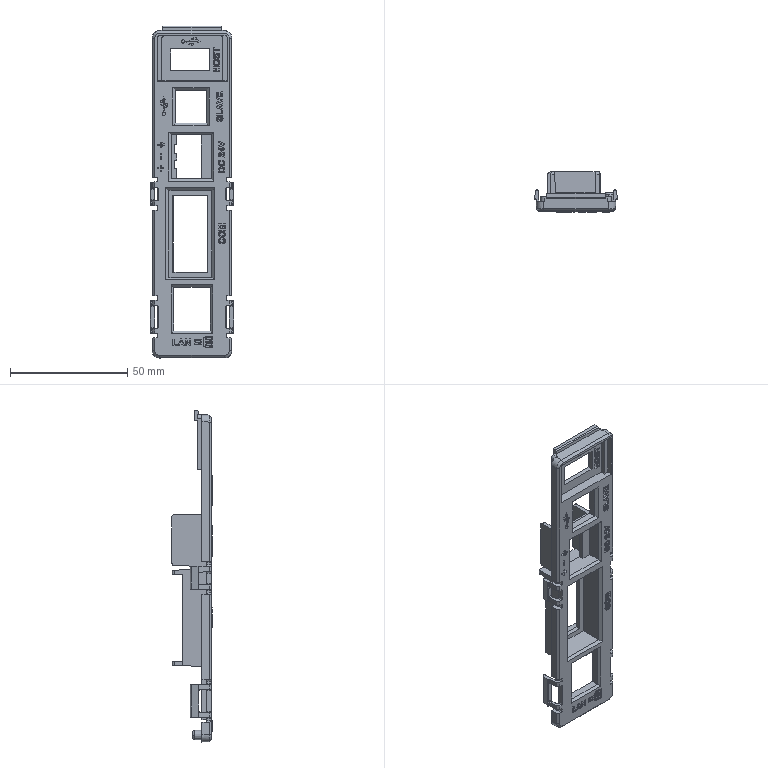Part | SolidWorks | features BaseBody 1 | 1 solid | 774 faces | box 35.585 x 17.1 x 141.528 mm | volume 13223 mm3 | plane 468 | spline 231 | cylinder 71 | cone 4 | commonest cylinder face diameters 1 x32 2 x21 0.6 x8 1.2 x4 6 x4 3 x2